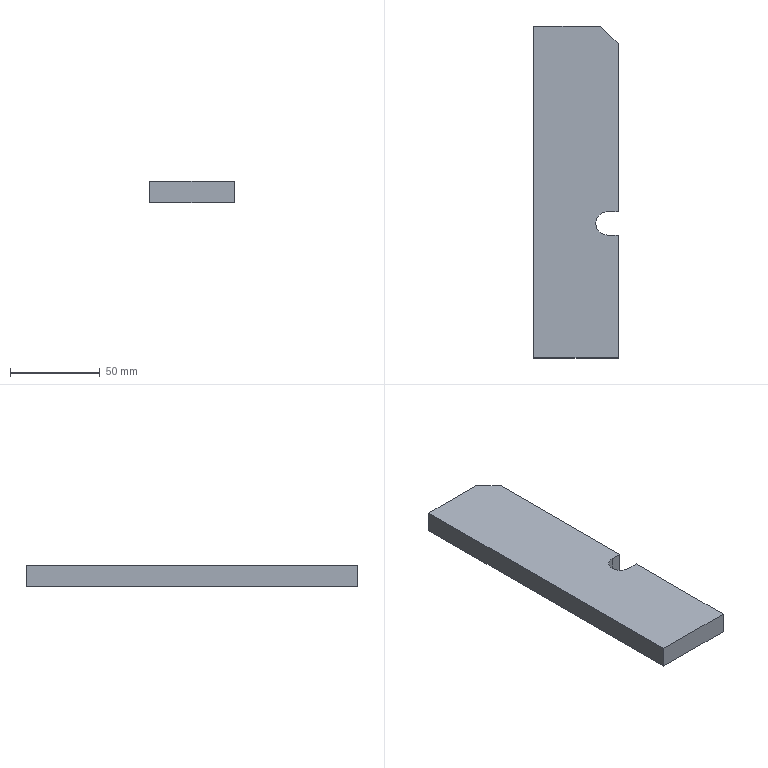Part | SolidWorks | features ICE 2, Chamfer 1, Extrusion 1, Fillet 1 | 1 solid | 12 faces | box 47 x 185 x 12 mm | volume 102008 mm3 | plane 10 | cylinder 2 | commonest cylinder face diameters 13 x2
STEP:
#1=CARTESIAN_POINT('',(34.5,75.,6.));
#2=VERTEX_POINT('',#1);
#3=CARTESIAN_POINT('',(41.,81.5,6.));
#4=VERTEX_POINT('',#3);
#5=CARTESIAN_POINT('',(41.,75.,6.));
#6=DIRECTION('',(0.,0.,-1.));
#7=DIRECTION('',(1.,0.,0.));
#8=AXIS2_PLACEMENT_3D('',#5,#6,#7);
#9=CIRCLE('',#8,6.5);
#10=EDGE_CURVE('',#2,#4,#9,.T.);
#11=ORIENTED_EDGE('',*,*,#10,.F.);
#12=CARTESIAN_POINT('',(34.5,75.,-6.));
#13=VERTEX_POINT('',#12);
#14=CARTESIAN_POINT('',(34.5,75.,6.001));
#15=DIRECTION('',(0.,0.,-1.));
#16=VECTOR('',#15,1000.);
#17=LINE('',#14,#16);
#18=EDGE_CURVE('',#2,#13,#17,.T.);
#19=ORIENTED_EDGE('',*,*,#18,.T.);
#20=CARTESIAN_POINT('',(41.,81.5,-6.));
#21=VERTEX_POINT('',#20);
#22=CARTESIAN_POINT('',(41.,75.,-6.));
#23=DIRECTION('',(0.,0.,-1.));
#24=DIRECTION('',(1.,0.,0.));
#25=AXIS2_PLACEMENT_3D('',#22,#23,#24);
#26=CIRCLE('',#25,6.5);
#27=EDGE_CURVE('',#13,#21,#26,.T.);
#28=ORIENTED_EDGE('',*,*,#27,.T.);
#29=CARTESIAN_POINT('',(41.,81.5,6.001));
#30=DIRECTION('',(0.,0.,-1.));
#31=VECTOR('',#30,1000.);
#32=LINE('',#29,#31);
#33=EDGE_CURVE('',#4,#21,#32,.T.);
#34=ORIENTED_EDGE('',*,*,#33,.F.);
#35=EDGE_LOOP('',(#11,#19,#28,#34));
#36=FACE_OUTER_BOUND('',#35,.T.);
#37=CARTESIAN_POINT('',(41.,75.,6.001));
#38=DIRECTION('',(0.,0.,-1.));
#39=DIRECTION('',(-1.,0.,0.));
#40=AXIS2_PLACEMENT_3D('',#37,#38,#39);
#41=CYLINDRICAL_SURFACE('',#40,6.5);
#42=ADVANCED_FACE('',(#36),#41,.F.);
#43=CARTESIAN_POINT('',(47.,81.5,6.));
#44=VERTEX_POINT('',#43);
#45=CARTESIAN_POINT('',(47.,175.,6.));
#46=VERTEX_POINT('',#45);
#47=CARTESIAN_POINT('',(47.,0.,6.));
#48=DIRECTION('',(0.,1.,0.));
#49=VECTOR('',#48,1000.);
#50=LINE('',#47,#49);
#51=EDGE_CURVE('',#44,#46,#50,.T.);
#52=ORIENTED_EDGE('',*,*,#51,.F.);
#53=CARTESIAN_POINT('',(47.,81.5,-6.));
#54=VERTEX_POINT('',#53);
#55=CARTESIAN_POINT('',(47.,81.5,6.001));
#56=DIRECTION('',(0.,0.,-1.));
#57=VECTOR('',#56,1000.);
#58=LINE('',#55,#57);
#59=EDGE_CURVE('',#44,#54,#58,.T.);
#60=ORIENTED_EDGE('',*,*,#59,.T.);
#61=CARTESIAN_POINT('',(47.,175.,-6.));
#62=VERTEX_POINT('',#61);
#63=CARTESIAN_POINT('',(47.,0.,-6.));
#64=DIRECTION('',(0.,1.,0.));
#65=VECTOR('',#64,1000.);
#66=LINE('',#63,#65);
#67=EDGE_CURVE('',#54,#62,#66,.T.);
#68=ORIENTED_EDGE('',*,*,#67,.T.);
#69=CARTESIAN_POINT('',(47.,175.,6.));
#70=DIRECTION('',(0.,0.,1.));
#71=VECTOR('',#70,1000.);
#72=LINE('',#69,#71);
#73=EDGE_CURVE('',#62,#46,#72,.T.);
#74=ORIENTED_EDGE('',*,*,#73,.T.);
#75=EDGE_LOOP('',(#52,#60,#68,#74));
#76=FACE_OUTER_BOUND('',#75,.T.);
#77=CARTESIAN_POINT('',(47.,0.,6.));
#78=DIRECTION('',(-1.,0.,0.));
#79=DIRECTION('',(0.,0.,1.));
#80=AXIS2_PLACEMENT_3D('',#77,#78,#79);
#81=PLANE('',#80);
#82=ADVANCED_FACE('',(#76),#81,.F.);
#83=CARTESIAN_POINT('',(0.,185.,-6.));
#84=VERTEX_POINT('',#83);
#85=CARTESIAN_POINT('',(0.,0.,-6.));
#86=VERTEX_POINT('',#85);
#87=CARTESIAN_POINT('',(0.,185.,-6.));
#88=DIRECTION('',(0.,-1.,0.));
#89=VECTOR('',#88,1000.);
#90=LINE('',#87,#89);
#91=EDGE_CURVE('',#84,#86,#90,.T.);
#92=ORIENTED_EDGE('',*,*,#91,.T.);
#93=CARTESIAN_POINT('',(0.,0.,6.));
#94=VERTEX_POINT('',#93);
#95=CARTESIAN_POINT('',(0.,0.,6.));
#96=DIRECTION('',(0.,0.,-1.));
#97=VECTOR('',#96,1000.);
#98=LINE('',#95,#97);
#99=EDGE_CURVE('',#94,#86,#98,.T.);
#100=ORIENTED_EDGE('',*,*,#99,.F.);
#101=CARTESIAN_POINT('',(0.,185.,6.));
#102=VERTEX_POINT('',#101);
#103=CARTESIAN_POINT('',(0.,185.,6.));
#104=DIRECTION('',(0.,-1.,0.));
#105=VECTOR('',#104,1000.);
#106=LINE('',#103,#105);
#107=EDGE_CURVE('',#102,#94,#106,.T.);
#108=ORIENTED_EDGE('',*,*,#107,.F.);
#109=CARTESIAN_POINT('',(0.,185.,6.));
#110=DIRECTION('',(0.,0.,-1.));
#111=VECTOR('',#110,1000.);
#112=LINE('',#109,#111);
#113=EDGE_CURVE('',#102,#84,#112,.T.);
#114=ORIENTED_EDGE('',*,*,#113,.T.);
#115=EDGE_LOOP('',(#92,#100,#108,#114));
#116=FACE_OUTER_BOUND('',#115,.T.);
#117=CARTESIAN_POINT('',(0.,185.,6.));
#118=DIRECTION('',(1.,0.,0.));
#119=DIRECTION('',(0.,0.,-1.));
#120=AXIS2_PLACEMENT_3D('',#117,#118,#119);
#121=PLANE('',#120);
#122=ADVANCED_FACE('',(#116),#121,.F.);
#123=CARTESIAN_POINT('',(47.,0.,-6.));
#124=VERTEX_POINT('',#123);
#125=CARTESIAN_POINT('',(0.,0.,-6.));
#126=DIRECTION('',(1.,0.,0.));
#127=VECTOR('',#126,1000.);
#128=LINE('',#125,#127);
#129=EDGE_CURVE('',#86,#124,#128,.T.);
#130=ORIENTED_EDGE('',*,*,#129,.T.);
#131=CARTESIAN_POINT('',(47.,0.,6.));
#132=VERTEX_POINT('',#131);
#133=CARTESIAN_POINT('',(47.,0.,6.));
#134=DIRECTION('',(0.,0.,-1.));
#135=VECTOR('',#134,1000.);
#136=LINE('',#133,#135);
#137=EDGE_CURVE('',#132,#124,#136,.T.);
#138=ORIENTED_EDGE('',*,*,#137,.F.);
#139=CARTESIAN_POINT('',(0.,0.,6.));
#140=DIRECTION('',(1.,0.,0.));
#141=VECTOR('',#140,1000.);
#142=LINE('',#139,#141);
#143=EDGE_CURVE('',#94,#132,#142,.T.);
#144=ORIENTED_EDGE('',*,*,#143,.F.);
#145=ORIENTED_EDGE('',*,*,#99,.T.);
#146=EDGE_LOOP('',(#130,#138,#144,#145));
#147=FACE_OUTER_BOUND('',#146,.T.);
#148=CARTESIAN_POINT('',(0.,0.,6.));
#149=DIRECTION('',(0.,1.,0.));
#150=DIRECTION('',(0.,0.,1.));
#151=AXIS2_PLACEMENT_3D('',#148,#149,#150);
#152=PLANE('',#151);
#153=ADVANCED_FACE('',(#147),#152,.F.);
#154=CARTESIAN_POINT('',(47.,68.5,-6.));
#155=VERTEX_POINT('',#154);
#156=CARTESIAN_POINT('',(47.,0.,-6.));
#157=DIRECTION('',(0.,1.,0.));
#158=VECTOR('',#157,1000.);
#159=LINE('',#156,#158);
#160=EDGE_CURVE('',#124,#155,#159,.T.);
#161=ORIENTED_EDGE('',*,*,#160,.T.);
#162=CARTESIAN_POINT('',(47.,68.5,6.));
#163=VERTEX_POINT('',#162);
#164=CARTESIAN_POINT('',(47.,68.5,6.001));
#165=DIRECTION('',(0.,0.,-1.));
#166=VECTOR('',#165,1000.);
#167=LINE('',#164,#166);
#168=EDGE_CURVE('',#163,#155,#167,.T.);
#169=ORIENTED_EDGE('',*,*,#168,.F.);
#170=CARTESIAN_POINT('',(47.,0.,6.));
#171=DIRECTION('',(0.,1.,0.));
#172=VECTOR('',#171,1000.);
#173=LINE('',#170,#172);
#174=EDGE_CURVE('',#132,#163,#173,.T.);
#175=ORIENTED_EDGE('',*,*,#174,.F.);
#176=ORIENTED_EDGE('',*,*,#137,.T.);
#177=EDGE_LOOP('',(#161,#169,#175,#176));
#178=FACE_OUTER_BOUND('',#177,.T.);
#179=CARTESIAN_POINT('',(47.,0.,6.));
#180=DIRECTION('',(-1.,0.,0.));
#181=DIRECTION('',(0.,0.,1.));
#182=AXIS2_PLACEMENT_3D('',#179,#180,#181);
#183=PLANE('',#182);
#184=ADVANCED_FACE('',(#178),#183,.F.);
#185=CARTESIAN_POINT('',(37.,185.,6.));
#186=VERTEX_POINT('',#185);
#187=CARTESIAN_POINT('',(47.,185.,6.));
#188=DIRECTION('',(-1.,0.,0.));
#189=VECTOR('',#188,1000.);
#190=LINE('',#187,#189);
#191=EDGE_CURVE('',#186,#102,#190,.T.);
#192=ORIENTED_EDGE('',*,*,#191,.F.);
#193=CARTESIAN_POINT('',(37.,185.,-6.));
#194=VERTEX_POINT('',#193);
#195=CARTESIAN_POINT('',(37.,185.,6.));
#196=DIRECTION('',(0.,0.,-1.));
#197=VECTOR('',#196,1000.);
#198=LINE('',#195,#197);
#199=EDGE_CURVE('',#186,#194,#198,.T.);
#200=ORIENTED_EDGE('',*,*,#199,.T.);
#201=CARTESIAN_POINT('',(47.,185.,-6.));
#202=DIRECTION('',(-1.,0.,0.));
#203=VECTOR('',#202,1000.);
#204=LINE('',#201,#203);
#205=EDGE_CURVE('',#194,#84,#204,.T.);
#206=ORIENTED_EDGE('',*,*,#205,.T.);
#207=ORIENTED_EDGE('',*,*,#113,.F.);
#208=EDGE_LOOP('',(#192,#200,#206,#207));
#209=FACE_OUTER_BOUND('',#208,.T.);
#210=CARTESIAN_POINT('',(47.,185.,6.));
#211=DIRECTION('',(0.,-1.,0.));
#212=DIRECTION('',(0.,0.,-1.));
#213=AXIS2_PLACEMENT_3D('',#210,#211,#212);
#214=PLANE('',#213);
#215=ADVANCED_FACE('',(#209),#214,.F.);
#216=CARTESIAN_POINT('',(47.,81.5,6.));
#217=DIRECTION('',(1.,0.,0.));
#218=VECTOR('',#217,1000.);
#219=LINE('',#216,#218);
#220=EDGE_CURVE('',#4,#44,#219,.T.);
#221=ORIENTED_EDGE('',*,*,#220,.T.);
#222=ORIENTED_EDGE('',*,*,#51,.T.);
#223=CARTESIAN_POINT('',(111.,111.,6.));
#224=DIRECTION('',(-0.7071,0.7071,0.));
#225=VECTOR('',#224,1000.);
#226=LINE('',#223,#225);
#227=EDGE_CURVE('',#46,#186,#226,.T.);
#228=ORIENTED_EDGE('',*,*,#227,.T.);
#229=ORIENTED_EDGE('',*,*,#191,.T.);
#230=ORIENTED_EDGE('',*,*,#107,.T.);
#231=ORIENTED_EDGE('',*,*,#143,.T.);
#232=ORIENTED_EDGE('',*,*,#174,.T.);
#233=CARTESIAN_POINT('',(41.,68.5,6.));
#234=VERTEX_POINT('',#233);
#235=CARTESIAN_POINT('',(41.,68.5,6.));
#236=DIRECTION('',(-1.,0.,0.));
#237=VECTOR('',#236,1000.);
#238=LINE('',#235,#237);
#239=EDGE_CURVE('',#163,#234,#238,.T.);
#240=ORIENTED_EDGE('',*,*,#239,.T.);
#241=CARTESIAN_POINT('',(41.,75.,6.));
#242=DIRECTION('',(0.,0.,-1.));
#243=DIRECTION('',(1.,0.,0.));
#244=AXIS2_PLACEMENT_3D('',#241,#242,#243);
#245=CIRCLE('',#244,6.5);
#246=EDGE_CURVE('',#234,#2,#245,.T.);
#247=ORIENTED_EDGE('',*,*,#246,.T.);
#248=ORIENTED_EDGE('',*,*,#10,.T.);
#249=EDGE_LOOP('',(#221,#222,#228,#229,#230,#231,#232,#240,#247,#248));
#250=FACE_OUTER_BOUND('',#249,.T.);
#251=CARTESIAN_POINT('',(0.,0.,6.));
#252=DIRECTION('',(0.,0.,1.));
#253=DIRECTION('',(1.,0.,0.));
#254=AXIS2_PLACEMENT_3D('',#251,#252,#253);
#255=PLANE('',#254);
#256=ADVANCED_FACE('',(#250),#255,.T.);
#257=ORIENTED_EDGE('',*,*,#67,.F.);
#258=CARTESIAN_POINT('',(47.,81.5,-6.));
#259=DIRECTION('',(1.,0.,0.));
#260=VECTOR('',#259,1000.);
#261=LINE('',#258,#260);
#262=EDGE_CURVE('',#21,#54,#261,.T.);
#263=ORIENTED_EDGE('',*,*,#262,.F.);
#264=ORIENTED_EDGE('',*,*,#27,.F.);
#265=CARTESIAN_POINT('',(41.,68.5,-6.));
#266=VERTEX_POINT('',#265);
#267=CARTESIAN_POINT('',(41.,75.,-6.));
#268=DIRECTION('',(0.,0.,-1.));
#269=DIRECTION('',(1.,0.,0.));
#270=AXIS2_PLACEMENT_3D('',#267,#268,#269);
#271=CIRCLE('',#270,6.5);
#272=EDGE_CURVE('',#266,#13,#271,.T.);
#273=ORIENTED_EDGE('',*,*,#272,.F.);
#274=CARTESIAN_POINT('',(41.,68.5,-6.));
#275=DIRECTION('',(-1.,0.,0.));
#276=VECTOR('',#275,1000.);
#277=LINE('',#274,#276);
#278=EDGE_CURVE('',#155,#266,#277,.T.);
#279=ORIENTED_EDGE('',*,*,#278,.F.);
#280=ORIENTED_EDGE('',*,*,#160,.F.);
#281=ORIENTED_EDGE('',*,*,#129,.F.);
#282=ORIENTED_EDGE('',*,*,#91,.F.);
#283=ORIENTED_EDGE('',*,*,#205,.F.);
#284=CARTESIAN_POINT('',(37.,185.,-6.));
#285=DIRECTION('',(0.7071,-0.7071,0.));
#286=VECTOR('',#285,1000.);
#287=LINE('',#284,#286);
#288=EDGE_CURVE('',#194,#62,#287,.T.);
#289=ORIENTED_EDGE('',*,*,#288,.T.);
#290=EDGE_LOOP('',(#257,#263,#264,#273,#279,#280,#281,#282,#283,#289));
#291=FACE_OUTER_BOUND('',#290,.T.);
#292=CARTESIAN_POINT('',(0.,0.,-6.));
#293=DIRECTION('',(0.,0.,1.));
#294=DIRECTION('',(1.,0.,0.));
#295=AXIS2_PLACEMENT_3D('',#292,#293,#294);
#296=PLANE('',#295);
#297=ADVANCED_FACE('',(#291),#296,.F.);
#298=ORIENTED_EDGE('',*,*,#227,.F.);
#299=ORIENTED_EDGE('',*,*,#73,.F.);
#300=ORIENTED_EDGE('',*,*,#288,.F.);
#301=ORIENTED_EDGE('',*,*,#199,.F.);
#302=EDGE_LOOP('',(#298,#299,#300,#301));
#303=FACE_OUTER_BOUND('',#302,.T.);
#304=CARTESIAN_POINT('',(37.,185.,6.));
#305=DIRECTION('',(-0.7071,-0.7071,0.));
#306=DIRECTION('',(0.,0.,-1.));
#307=AXIS2_PLACEMENT_3D('',#304,#305,#306);
#308=PLANE('',#307);
#309=ADVANCED_FACE('',(#303),#308,.F.);
#310=ORIENTED_EDGE('',*,*,#33,.T.);
#311=ORIENTED_EDGE('',*,*,#262,.T.);
#312=ORIENTED_EDGE('',*,*,#59,.F.);
#313=ORIENTED_EDGE('',*,*,#220,.F.);
#314=EDGE_LOOP('',(#310,#311,#312,#313));
#315=FACE_OUTER_BOUND('',#314,.T.);
#316=CARTESIAN_POINT('',(47.,81.5,6.001));
#317=DIRECTION('',(0.,1.,0.));
#318=DIRECTION('',(-1.,0.,0.));
#319=AXIS2_PLACEMENT_3D('',#316,#317,#318);
#320=PLANE('',#319);
#321=ADVANCED_FACE('',(#315),#320,.F.);
#322=ORIENTED_EDGE('',*,*,#18,.F.);
#323=ORIENTED_EDGE('',*,*,#246,.F.);
#324=CARTESIAN_POINT('',(41.,68.5,6.001));
#325=DIRECTION('',(0.,0.,-1.));
#326=VECTOR('',#325,1000.);
#327=LINE('',#324,#326);
#328=EDGE_CURVE('',#234,#266,#327,.T.);
#329=ORIENTED_EDGE('',*,*,#328,.T.);
#330=ORIENTED_EDGE('',*,*,#272,.T.);
#331=EDGE_LOOP('',(#322,#323,#329,#330));
#332=FACE_OUTER_BOUND('',#331,.T.);
#333=CARTESIAN_POINT('',(41.,75.,6.001));
#334=DIRECTION('',(0.,0.,-1.));
#335=DIRECTION('',(-1.,0.,0.));
#336=AXIS2_PLACEMENT_3D('',#333,#334,#335);
#337=CYLINDRICAL_SURFACE('',#336,6.5);
#338=ADVANCED_FACE('',(#332),#337,.F.);
#339=ORIENTED_EDGE('',*,*,#168,.T.);
#340=ORIENTED_EDGE('',*,*,#278,.T.);
#341=ORIENTED_EDGE('',*,*,#328,.F.);
#342=ORIENTED_EDGE('',*,*,#239,.F.);
#343=EDGE_LOOP('',(#339,#340,#341,#342));
#344=FACE_OUTER_BOUND('',#343,.T.);
#345=CARTESIAN_POINT('',(41.,68.5,6.001));
#346=DIRECTION('',(0.,-1.,0.));
#347=DIRECTION('',(0.,0.,-1.));
#348=AXIS2_PLACEMENT_3D('',#345,#346,#347);
#349=PLANE('',#348);
#350=ADVANCED_FACE('',(#344),#349,.F.);
#351=CLOSED_SHELL('',(#42,#82,#122,#153,#184,#215,#256,#297,#309,#321,#338,#350));
#352=MANIFOLD_SOLID_BREP('',#351);
#353=CARTESIAN_POINT('',(0.,0.,0.));
#354=DIRECTION('',(0.,0.,1.));
#355=DIRECTION('',(1.,0.,0.));
#356=AXIS2_PLACEMENT_3D('',#353,#354,#355);
#357=(LENGTH_UNIT()NAMED_UNIT(*)SI_UNIT(.MILLI.,.METRE.));
#358=UNCERTAINTY_MEASURE_WITH_UNIT(LENGTH_MEASURE(0.00001),#357,'','');
#359=(NAMED_UNIT(*)PLANE_ANGLE_UNIT()SI_UNIT($,.RADIAN.));
#360=(NAMED_UNIT(*)SI_UNIT($,.STERADIAN.)SOLID_ANGLE_UNIT());
#361=(GEOMETRIC_REPRESENTATION_CONTEXT(3)GLOBAL_UNCERTAINTY_ASSIGNED_CONTEXT((#358))GLOBAL_UNIT_ASSIGNED_CONTEXT((#357,#359,#360))REPRESENTATION_CONTEXT('',''));
#362=ADVANCED_BREP_SHAPE_REPRESENTATION('',(#352,#356),#361);